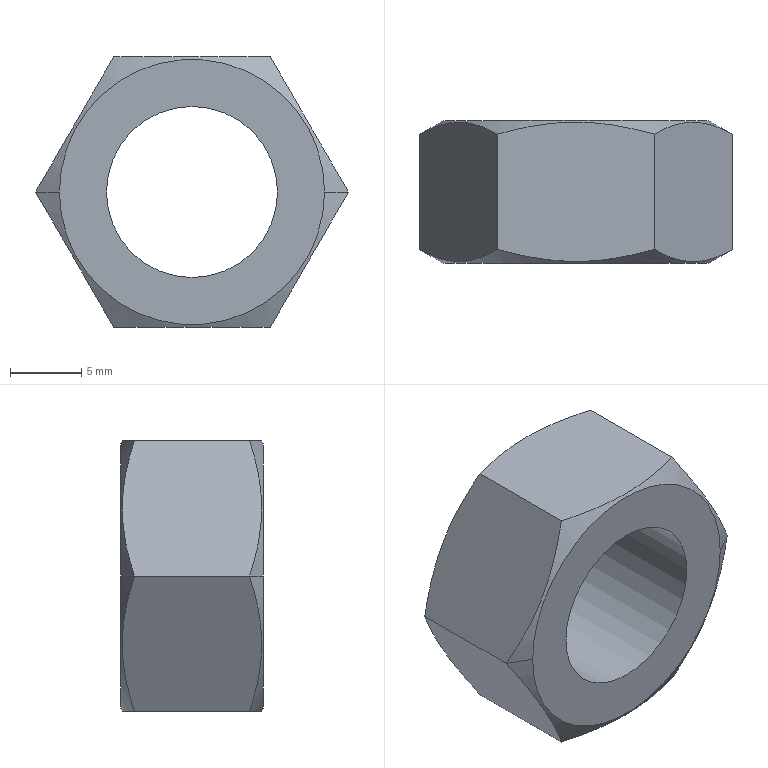Part | STEP file | LIB_27044255_HEX_NUT_M12_SIMPLE | 1 solid | 14 faces | box 21.939 x 10 x 19 mm | volume 1972 mm3 | plane 8 | cone 4 | cylinder 2 | commonest cylinder face diameters 12 x2